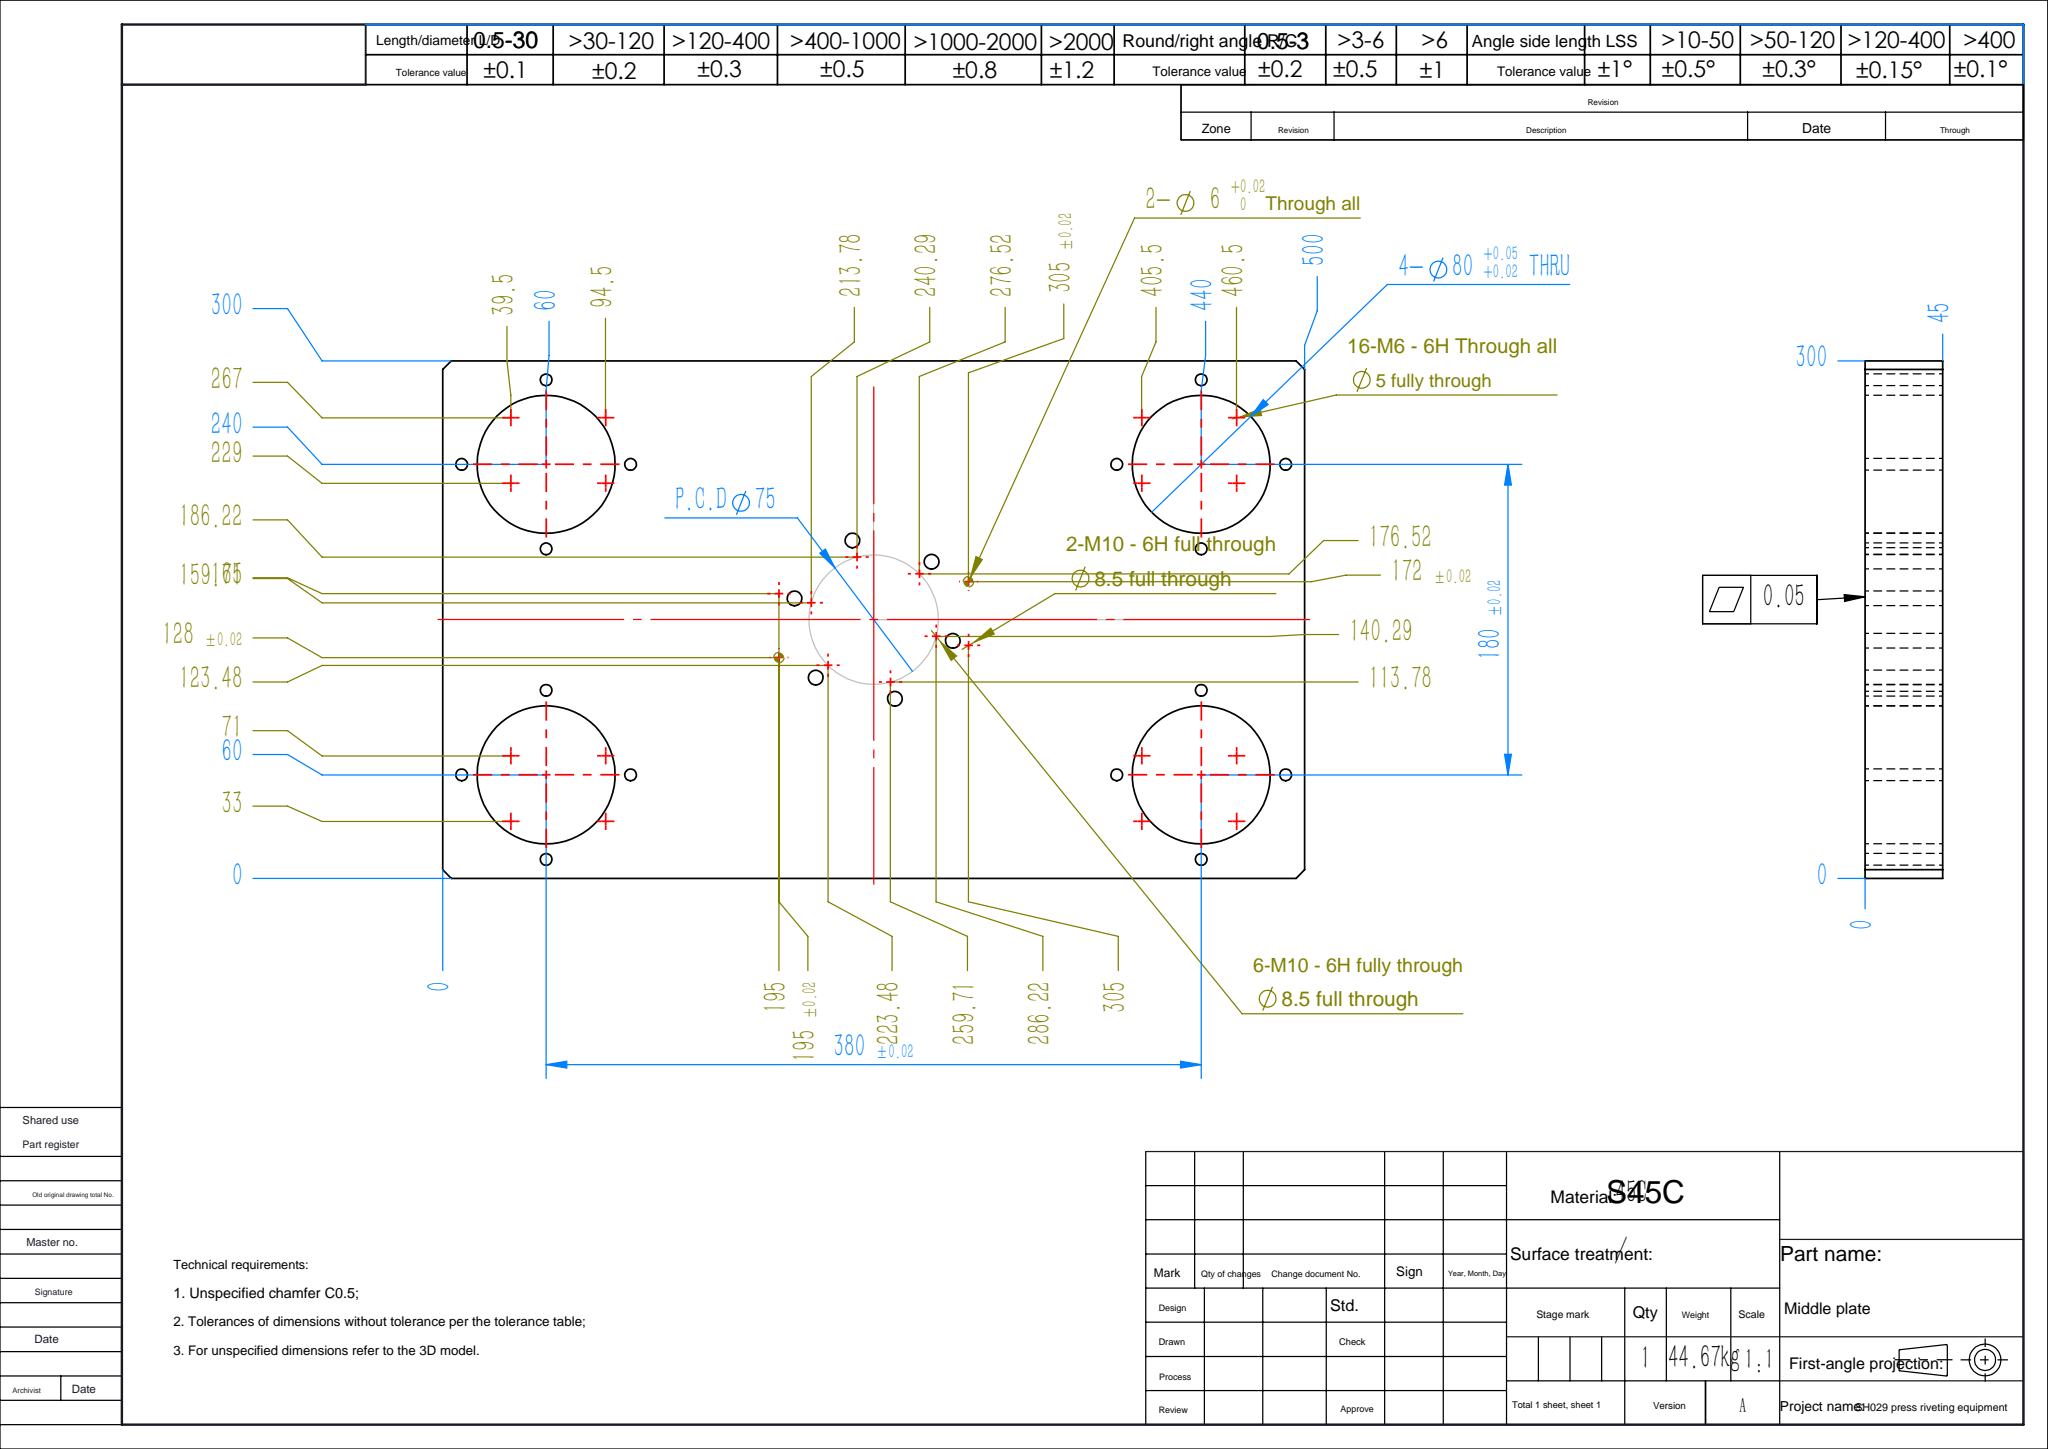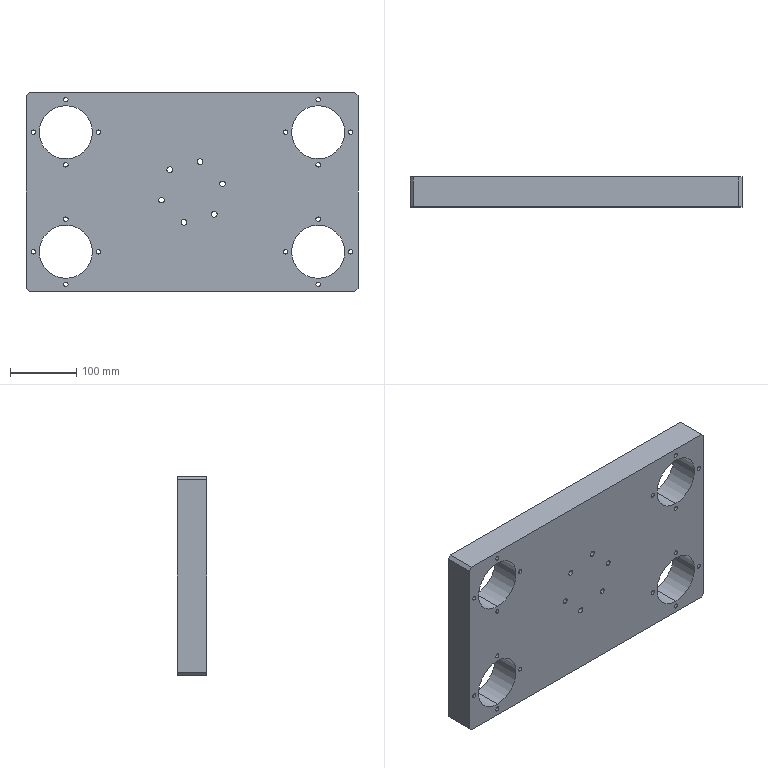Part | SolidWorks | features HoleWzd 2, Chamfer 1, Cut 1, Extrusion 1 | 1 solid | 62 faces | box 500 x 45 x 300 mm | volume 5801502 mm3 | cylinder 52 | plane 10 | commonest cylinder face diameters 6.8 x32 8.5 x12 80 x8